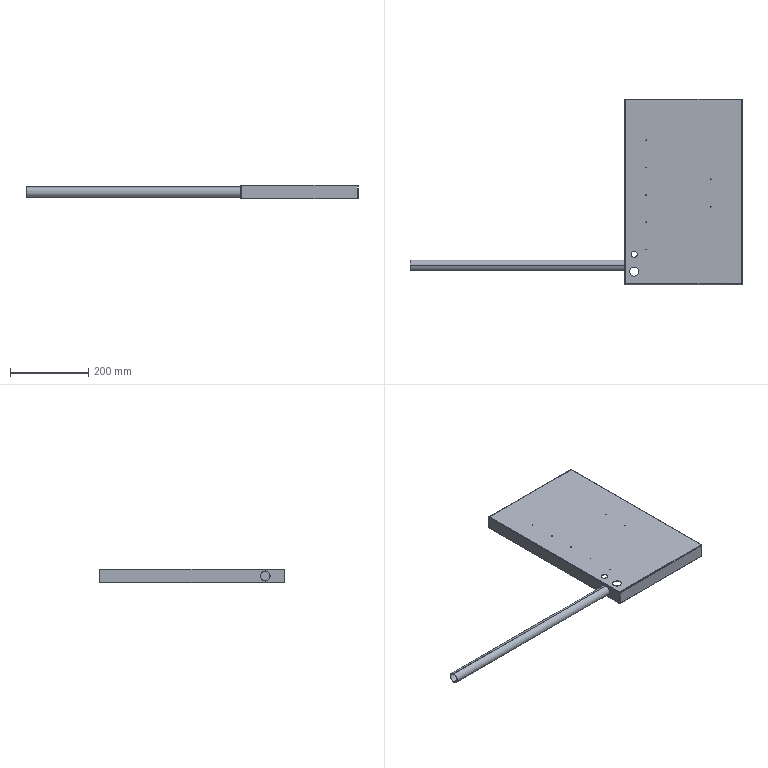Part | 1 solid | 69 faces | box 850 x 475 x 35 mm | volume 278714 mm3 | cylinder 32 | plane 29 | spline 8 | commonest cylinder face diameters 2 x14 1.473 x5 3.873 x5 16 x2 23 x2 24 x2